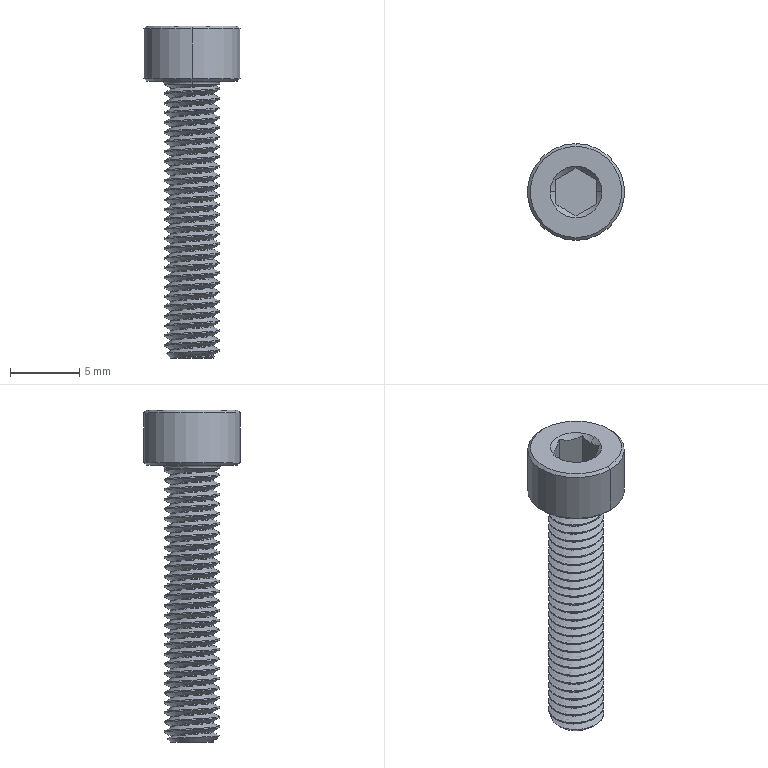Part | NX | features solid 2 | 1 solid | 85 faces | box 7 x 7 x 24 mm | volume 328.793 mm3 | cylinder 58 | cone 12 | plane 10 | spline 3 | torus 2 | commonest cylinder face diameters 4 x56 7 x2